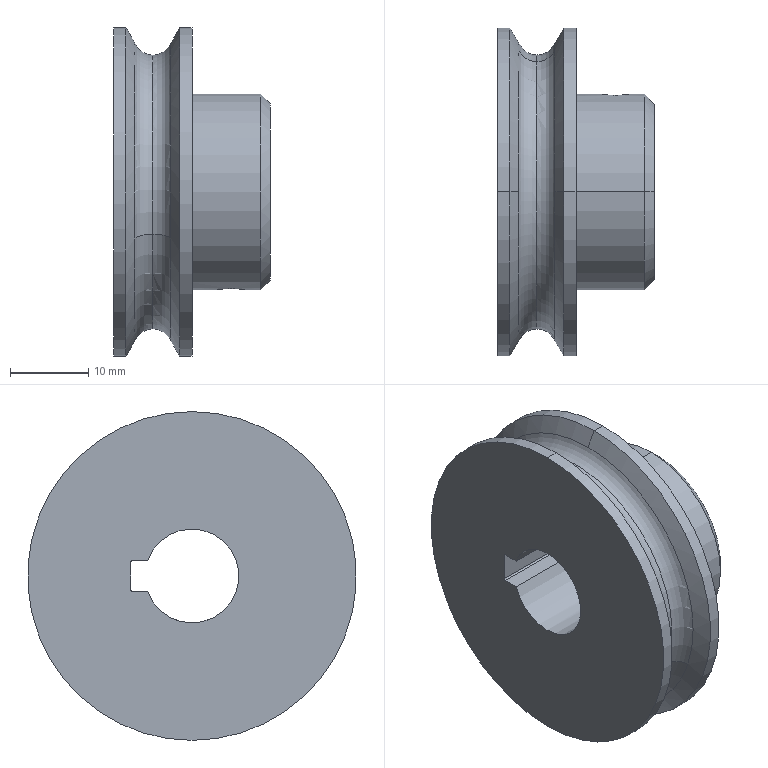Part | STEP file | MT-COMBO-119-S022 | 1 solid | 33 faces | box 20 x 42 x 42 mm | volume 14178 mm3 | cylinder 13 | cone 10 | plane 6 | torus 4 | commonest cylinder face diameters 3.242 x4 42 x4 0.4 x2 25 x2 12 x1
STEP:
#1=CARTESIAN_POINT('',(0.,16.643,5.408));
#2=VERTEX_POINT('',#1);
#3=CARTESIAN_POINT('',(2.299,18.087,5.877));
#4=VERTEX_POINT('',#3);
#5=CARTESIAN_POINT('',(0.,19.021,6.18));
#6=DIRECTION('',(0.,-0.309,0.9511));
#7=DIRECTION('',(-0.9196,-0.3736,-0.1214));
#8=AXIS2_PLACEMENT_3D('',#5,#6,#7);
#9=CIRCLE('',#8,2.5);
#10=EDGE_CURVE('',#2,#4,#9,.T.);
#11=ORIENTED_EDGE('',*,*,#10,.F.);
#12=CARTESIAN_POINT('',(0.,-16.643,-5.408));
#13=VERTEX_POINT('',#12);
#14=CARTESIAN_POINT('',(0.,0.,0.));
#15=DIRECTION('',(1.,0.,0.));
#16=DIRECTION('',(0.,0.,-1.));
#17=AXIS2_PLACEMENT_3D('',#14,#15,#16);
#18=CIRCLE('',#17,17.5);
#19=EDGE_CURVE('',#2,#13,#18,.T.);
#20=ORIENTED_EDGE('',*,*,#19,.T.);
#21=CARTESIAN_POINT('',(2.299,-18.087,-5.877));
#22=VERTEX_POINT('',#21);
#23=CARTESIAN_POINT('',(0.,-19.021,-6.18));
#24=DIRECTION('',(0.,0.309,-0.9511));
#25=DIRECTION('',(-0.9196,0.3736,0.1214));
#26=AXIS2_PLACEMENT_3D('',#23,#24,#25);
#27=CIRCLE('',#26,2.5);
#28=EDGE_CURVE('',#13,#22,#27,.T.);
#29=ORIENTED_EDGE('',*,*,#28,.T.);
#30=CARTESIAN_POINT('',(2.299,0.,19.018));
#31=VERTEX_POINT('',#30);
#32=CARTESIAN_POINT('',(2.299,0.,0.));
#33=DIRECTION('',(1.,0.,0.));
#34=DIRECTION('',(0.,0.,-1.));
#35=AXIS2_PLACEMENT_3D('',#32,#33,#34);
#36=CIRCLE('',#35,19.018);
#37=EDGE_CURVE('',#31,#22,#36,.T.);
#38=ORIENTED_EDGE('',*,*,#37,.F.);
#39=CARTESIAN_POINT('',(2.299,0.,0.));
#40=DIRECTION('',(1.,0.,0.));
#41=DIRECTION('',(0.,0.,-1.));
#42=AXIS2_PLACEMENT_3D('',#39,#40,#41);
#43=CIRCLE('',#42,19.018);
#44=EDGE_CURVE('',#4,#31,#43,.T.);
#45=ORIENTED_EDGE('',*,*,#44,.F.);
#46=EDGE_LOOP('',(#11,#20,#29,#38,#45));
#47=FACE_OUTER_BOUND('',#46,.T.);
#48=CARTESIAN_POINT('',(0.,0.,0.));
#49=DIRECTION('',(1.,0.,0.));
#50=DIRECTION('',(0.,0.309,-0.9511));
#51=AXIS2_PLACEMENT_3D('',#48,#49,#50);
#52=TOROIDAL_SURFACE('',#51,20.,2.5);
#53=ADVANCED_FACE('',(#47),#52,.F.);
#54=ORIENTED_EDGE('',*,*,#28,.F.);
#55=CARTESIAN_POINT('',(0.,0.,0.));
#56=DIRECTION('',(1.,0.,0.));
#57=DIRECTION('',(0.,0.,-1.));
#58=AXIS2_PLACEMENT_3D('',#55,#56,#57);
#59=CIRCLE('',#58,17.5);
#60=EDGE_CURVE('',#13,#2,#59,.T.);
#61=ORIENTED_EDGE('',*,*,#60,.T.);
#62=ORIENTED_EDGE('',*,*,#10,.T.);
#63=CARTESIAN_POINT('',(2.299,0.,-19.018));
#64=VERTEX_POINT('',#63);
#65=CARTESIAN_POINT('',(2.299,0.,0.));
#66=DIRECTION('',(1.,0.,0.));
#67=DIRECTION('',(0.,0.,-1.));
#68=AXIS2_PLACEMENT_3D('',#65,#66,#67);
#69=CIRCLE('',#68,19.018);
#70=EDGE_CURVE('',#64,#4,#69,.T.);
#71=ORIENTED_EDGE('',*,*,#70,.F.);
#72=CARTESIAN_POINT('',(2.299,0.,0.));
#73=DIRECTION('',(1.,0.,0.));
#74=DIRECTION('',(0.,0.,-1.));
#75=AXIS2_PLACEMENT_3D('',#72,#73,#74);
#76=CIRCLE('',#75,19.018);
#77=EDGE_CURVE('',#22,#64,#76,.T.);
#78=ORIENTED_EDGE('',*,*,#77,.F.);
#79=EDGE_LOOP('',(#54,#61,#62,#71,#78));
#80=FACE_OUTER_BOUND('',#79,.T.);
#81=CARTESIAN_POINT('',(0.,0.,0.));
#82=DIRECTION('',(1.,0.,0.));
#83=DIRECTION('',(0.,-0.309,0.9511));
#84=AXIS2_PLACEMENT_3D('',#81,#82,#83);
#85=TOROIDAL_SURFACE('',#84,20.,2.5);
#86=ADVANCED_FACE('',(#80),#85,.F.);
#87=CARTESIAN_POINT('',(5.,0.,12.5));
#88=VERTEX_POINT('',#87);
#89=CARTESIAN_POINT('',(13.75,0.,12.5));
#90=VERTEX_POINT('',#89);
#91=CARTESIAN_POINT('',(5.,0.,12.5));
#92=DIRECTION('',(1.,0.,0.));
#93=VECTOR('',#92,1000.);
#94=LINE('',#91,#93);
#95=EDGE_CURVE('',#88,#90,#94,.T.);
#96=ORIENTED_EDGE('',*,*,#95,.F.);
#97=CARTESIAN_POINT('',(5.,0.,-12.5));
#98=VERTEX_POINT('',#97);
#99=CARTESIAN_POINT('',(5.,0.,0.));
#100=DIRECTION('',(1.,0.,0.));
#101=DIRECTION('',(0.,0.,-1.));
#102=AXIS2_PLACEMENT_3D('',#99,#100,#101);
#103=CIRCLE('',#102,12.5);
#104=EDGE_CURVE('',#88,#98,#103,.T.);
#105=ORIENTED_EDGE('',*,*,#104,.T.);
#106=CARTESIAN_POINT('',(8.,0.,-12.5));
#107=VERTEX_POINT('',#106);
#108=CARTESIAN_POINT('',(5.,0.,-12.5));
#109=DIRECTION('',(1.,0.,0.));
#110=VECTOR('',#109,1000.);
#111=LINE('',#108,#110);
#112=EDGE_CURVE('',#98,#107,#111,.T.);
#113=ORIENTED_EDGE('',*,*,#112,.T.);
#114=CARTESIAN_POINT('',(8.634,-1.357,-12.426));
#115=VERTEX_POINT('',#114);
#116=CARTESIAN_POINT('',(8.,0.,-12.5));
#117=CARTESIAN_POINT('',(8.,-0.2576,-12.5));
#118=CARTESIAN_POINT('',(8.059,-0.5152,-12.492));
#119=CARTESIAN_POINT('',(8.28,-0.9815,-12.464));
#120=CARTESIAN_POINT('',(8.441,-1.189,-12.444));
#121=CARTESIAN_POINT('',(8.634,-1.357,-12.426));
#122=B_SPLINE_CURVE_WITH_KNOTS('',3,(#116,#117,#118,#119,#120,#121),.UNSPECIFIED.,.F.,.F.,(4,2,4),(0.8726,0.9363,1.),.UNSPECIFIED.);
#123=EDGE_CURVE('',#107,#115,#122,.T.);
#124=ORIENTED_EDGE('',*,*,#123,.T.);
#125=CARTESIAN_POINT('',(12.,0.,-12.5));
#126=VERTEX_POINT('',#125);
#127=CARTESIAN_POINT('',(8.634,-1.357,-12.426));
#128=CARTESIAN_POINT('',(8.916,-1.603,-12.399));
#129=CARTESIAN_POINT('',(9.272,-1.767,-12.375));
#130=CARTESIAN_POINT('',(10.014,-1.894,-12.356));
#131=CARTESIAN_POINT('',(10.402,-1.857,-12.362));
#132=CARTESIAN_POINT('',(10.931,-1.655,-12.39));
#133=CARTESIAN_POINT('',(11.098,-1.565,-12.402));
#134=CARTESIAN_POINT('',(11.399,-1.34,-12.429));
#135=CARTESIAN_POINT('',(11.535,-1.205,-12.443));
#136=CARTESIAN_POINT('',(11.758,-0.904,-12.468));
#137=CARTESIAN_POINT('',(11.848,-0.7339,-12.48));
#138=CARTESIAN_POINT('',(11.969,-0.3777,-12.496));
#139=CARTESIAN_POINT('',(12.,-0.1886,-12.5));
#140=CARTESIAN_POINT('',(12.,0.,-12.5));
#141=B_SPLINE_CURVE_WITH_KNOTS('',3,(#127,#128,#129,#130,#131,#132,#133,#134,#135,#136,#137,#138,#139,#140),.UNSPECIFIED.,.F.,.F.,(4,2,2,2,2,2,4),(0.,0.09314,0.1863,0.2328,0.2794,0.326,0.3726),.UNSPECIFIED.);
#142=EDGE_CURVE('',#115,#126,#141,.T.);
#143=ORIENTED_EDGE('',*,*,#142,.T.);
#144=CARTESIAN_POINT('',(13.75,0.,-12.5));
#145=VERTEX_POINT('',#144);
#146=CARTESIAN_POINT('',(12.,0.,-12.5));
#147=DIRECTION('',(1.,0.,0.));
#148=VECTOR('',#147,1000.);
#149=LINE('',#146,#148);
#150=EDGE_CURVE('',#126,#145,#149,.T.);
#151=ORIENTED_EDGE('',*,*,#150,.T.);
#152=CARTESIAN_POINT('',(13.75,0.,0.));
#153=DIRECTION('',(1.,0.,0.));
#154=DIRECTION('',(0.,0.,-1.));
#155=AXIS2_PLACEMENT_3D('',#152,#153,#154);
#156=CIRCLE('',#155,12.5);
#157=EDGE_CURVE('',#90,#145,#156,.T.);
#158=ORIENTED_EDGE('',*,*,#157,.F.);
#159=EDGE_LOOP('',(#96,#105,#113,#124,#143,#151,#158));
#160=FACE_OUTER_BOUND('',#159,.T.);
#161=CARTESIAN_POINT('',(15.,0.,0.));
#162=DIRECTION('',(1.,0.,0.));
#163=DIRECTION('',(0.,1.,0.));
#164=AXIS2_PLACEMENT_3D('',#161,#162,#163);
#165=CYLINDRICAL_SURFACE('',#164,12.5);
#166=ADVANCED_FACE('',(#160),#165,.T.);
#167=CARTESIAN_POINT('',(15.,0.,-11.25));
#168=VERTEX_POINT('',#167);
#169=CARTESIAN_POINT('',(15.,0.,-11.25));
#170=DIRECTION('',(-0.7071,0.,-0.7071));
#171=VECTOR('',#170,1000.);
#172=LINE('',#169,#171);
#173=EDGE_CURVE('',#168,#145,#172,.T.);
#174=ORIENTED_EDGE('',*,*,#173,.F.);
#175=CARTESIAN_POINT('',(15.,0.,11.25));
#176=VERTEX_POINT('',#175);
#177=CARTESIAN_POINT('',(15.,0.,0.));
#178=DIRECTION('',(1.,0.,0.));
#179=DIRECTION('',(0.,0.,-1.));
#180=AXIS2_PLACEMENT_3D('',#177,#178,#179);
#181=CIRCLE('',#180,11.25);
#182=EDGE_CURVE('',#176,#168,#181,.T.);
#183=ORIENTED_EDGE('',*,*,#182,.F.);
#184=CARTESIAN_POINT('',(15.,0.,11.25));
#185=DIRECTION('',(-0.7071,0.,0.7071));
#186=VECTOR('',#185,1000.);
#187=LINE('',#184,#186);
#188=EDGE_CURVE('',#176,#90,#187,.T.);
#189=ORIENTED_EDGE('',*,*,#188,.T.);
#190=ORIENTED_EDGE('',*,*,#157,.T.);
#191=EDGE_LOOP('',(#174,#183,#189,#190));
#192=FACE_OUTER_BOUND('',#191,.T.);
#193=CARTESIAN_POINT('',(15.,0.,0.));
#194=DIRECTION('',(-1.,0.,0.));
#195=DIRECTION('',(0.,1.,0.));
#196=AXIS2_PLACEMENT_3D('',#193,#194,#195);
#197=CONICAL_SURFACE('',#196,11.25,0.7854);
#198=ADVANCED_FACE('',(#192),#197,.T.);
#199=ORIENTED_EDGE('',*,*,#173,.T.);
#200=CARTESIAN_POINT('',(13.75,0.,0.));
#201=DIRECTION('',(1.,0.,0.));
#202=DIRECTION('',(0.,0.,-1.));
#203=AXIS2_PLACEMENT_3D('',#200,#201,#202);
#204=CIRCLE('',#203,12.5);
#205=EDGE_CURVE('',#145,#90,#204,.T.);
#206=ORIENTED_EDGE('',*,*,#205,.T.);
#207=ORIENTED_EDGE('',*,*,#188,.F.);
#208=CARTESIAN_POINT('',(15.,0.,0.));
#209=DIRECTION('',(1.,0.,0.));
#210=DIRECTION('',(0.,0.,-1.));
#211=AXIS2_PLACEMENT_3D('',#208,#209,#210);
#212=CIRCLE('',#211,11.25);
#213=EDGE_CURVE('',#168,#176,#212,.T.);
#214=ORIENTED_EDGE('',*,*,#213,.F.);
#215=EDGE_LOOP('',(#199,#206,#207,#214));
#216=FACE_OUTER_BOUND('',#215,.T.);
#217=CARTESIAN_POINT('',(15.,0.,0.));
#218=DIRECTION('',(-1.,0.,0.));
#219=DIRECTION('',(0.,-1.,0.));
#220=AXIS2_PLACEMENT_3D('',#217,#218,#219);
#221=CONICAL_SURFACE('',#220,11.25,0.7854);
#222=ADVANCED_FACE('',(#216),#221,.T.);
#223=ORIENTED_EDGE('',*,*,#213,.T.);
#224=ORIENTED_EDGE('',*,*,#182,.T.);
#225=EDGE_LOOP('',(#223,#224));
#226=FACE_OUTER_BOUND('',#225,.T.);
#227=CARTESIAN_POINT('',(15.,5.657,2.));
#228=VERTEX_POINT('',#227);
#229=CARTESIAN_POINT('',(15.,5.657,-2.));
#230=VERTEX_POINT('',#229);
#231=CARTESIAN_POINT('',(15.,0.,0.));
#232=DIRECTION('',(1.,0.,0.));
#233=DIRECTION('',(0.,0.,-1.));
#234=AXIS2_PLACEMENT_3D('',#231,#232,#233);
#235=CIRCLE('',#234,6.);
#236=EDGE_CURVE('',#228,#230,#235,.T.);
#237=ORIENTED_EDGE('',*,*,#236,.F.);
#238=CARTESIAN_POINT('',(15.,7.6,2.));
#239=VERTEX_POINT('',#238);
#240=CARTESIAN_POINT('',(15.,6.,2.));
#241=DIRECTION('',(0.,1.,0.));
#242=VECTOR('',#241,1000.);
#243=LINE('',#240,#242);
#244=EDGE_CURVE('',#228,#239,#243,.T.);
#245=ORIENTED_EDGE('',*,*,#244,.T.);
#246=CARTESIAN_POINT('',(15.,7.8,1.8));
#247=VERTEX_POINT('',#246);
#248=CARTESIAN_POINT('',(15.,7.6,1.8));
#249=DIRECTION('',(-1.,0.,0.));
#250=DIRECTION('',(0.,0.,-1.));
#251=AXIS2_PLACEMENT_3D('',#248,#249,#250);
#252=CIRCLE('',#251,0.2);
#253=EDGE_CURVE('',#239,#247,#252,.T.);
#254=ORIENTED_EDGE('',*,*,#253,.T.);
#255=CARTESIAN_POINT('',(15.,7.8,-1.8));
#256=VERTEX_POINT('',#255);
#257=CARTESIAN_POINT('',(15.,7.8,0.));
#258=DIRECTION('',(0.,0.,-1.));
#259=VECTOR('',#258,1000.);
#260=LINE('',#257,#259);
#261=EDGE_CURVE('',#247,#256,#260,.T.);
#262=ORIENTED_EDGE('',*,*,#261,.T.);
#263=CARTESIAN_POINT('',(15.,7.6,-2.));
#264=VERTEX_POINT('',#263);
#265=CARTESIAN_POINT('',(15.,7.6,-1.8));
#266=DIRECTION('',(-1.,0.,0.));
#267=DIRECTION('',(0.,0.,-1.));
#268=AXIS2_PLACEMENT_3D('',#265,#266,#267);
#269=CIRCLE('',#268,0.2);
#270=EDGE_CURVE('',#256,#264,#269,.T.);
#271=ORIENTED_EDGE('',*,*,#270,.T.);
#272=CARTESIAN_POINT('',(15.,6.,-2.));
#273=DIRECTION('',(0.,-1.,0.));
#274=VECTOR('',#273,1000.);
#275=LINE('',#272,#274);
#276=EDGE_CURVE('',#264,#230,#275,.T.);
#277=ORIENTED_EDGE('',*,*,#276,.T.);
#278=EDGE_LOOP('',(#237,#245,#254,#262,#271,#277));
#279=FACE_BOUND('',#278,.T.);
#280=CARTESIAN_POINT('',(15.,6.,0.));
#281=DIRECTION('',(1.,0.,0.));
#282=DIRECTION('',(0.,0.,-1.));
#283=AXIS2_PLACEMENT_3D('',#280,#281,#282);
#284=PLANE('',#283);
#285=ADVANCED_FACE('',(#226,#279),#284,.T.);
#286=ORIENTED_EDGE('',*,*,#276,.F.);
#287=CARTESIAN_POINT('',(-5.,7.6,-2.));
#288=VERTEX_POINT('',#287);
#289=CARTESIAN_POINT('',(25.,7.6,-2.));
#290=DIRECTION('',(-1.,0.,0.));
#291=VECTOR('',#290,1000.);
#292=LINE('',#289,#291);
#293=EDGE_CURVE('',#264,#288,#292,.T.);
#294=ORIENTED_EDGE('',*,*,#293,.T.);
#295=CARTESIAN_POINT('',(-5.,5.657,-2.));
#296=VERTEX_POINT('',#295);
#297=CARTESIAN_POINT('',(-5.,4.2,-2.));
#298=DIRECTION('',(0.,1.,0.));
#299=VECTOR('',#298,1000.);
#300=LINE('',#297,#299);
#301=EDGE_CURVE('',#296,#288,#300,.T.);
#302=ORIENTED_EDGE('',*,*,#301,.F.);
#303=CARTESIAN_POINT('',(15.,5.657,-2.));
#304=DIRECTION('',(-1.,0.,0.));
#305=VECTOR('',#304,1000.);
#306=LINE('',#303,#305);
#307=EDGE_CURVE('',#230,#296,#306,.T.);
#308=ORIENTED_EDGE('',*,*,#307,.F.);
#309=EDGE_LOOP('',(#286,#294,#302,#308));
#310=FACE_OUTER_BOUND('',#309,.T.);
#311=CARTESIAN_POINT('',(25.,4.2,-2.));
#312=DIRECTION('',(0.,0.,1.));
#313=DIRECTION('',(1.,0.,0.));
#314=AXIS2_PLACEMENT_3D('',#311,#312,#313);
#315=PLANE('',#314);
#316=ADVANCED_FACE('',(#310),#315,.T.);
#317=CARTESIAN_POINT('',(-5.,5.657,2.));
#318=VERTEX_POINT('',#317);
#319=CARTESIAN_POINT('',(-5.,0.,0.));
#320=DIRECTION('',(1.,0.,0.));
#321=DIRECTION('',(0.,0.,-1.));
#322=AXIS2_PLACEMENT_3D('',#319,#320,#321);
#323=CIRCLE('',#322,6.);
#324=EDGE_CURVE('',#318,#296,#323,.T.);
#325=ORIENTED_EDGE('',*,*,#324,.F.);
#326=CARTESIAN_POINT('',(15.,5.657,2.));
#327=DIRECTION('',(1.,0.,0.));
#328=VECTOR('',#327,1000.);
#329=LINE('',#326,#328);
#330=EDGE_CURVE('',#318,#228,#329,.T.);
#331=ORIENTED_EDGE('',*,*,#330,.T.);
#332=ORIENTED_EDGE('',*,*,#236,.T.);
#333=ORIENTED_EDGE('',*,*,#307,.T.);
#334=EDGE_LOOP('',(#325,#331,#332,#333));
#335=FACE_OUTER_BOUND('',#334,.T.);
#336=CARTESIAN_POINT('',(11.621,0.,-6.));
#337=VERTEX_POINT('',#336);
#338=CARTESIAN_POINT('',(8.379,0.,-6.));
#339=VERTEX_POINT('',#338);
#340=CARTESIAN_POINT('',(11.621,0.,-6.));
#341=CARTESIAN_POINT('',(11.621,-0.2122,-6.));
#342=CARTESIAN_POINT('',(11.578,-0.4261,-5.988));
#343=CARTESIAN_POINT('',(11.415,-0.8177,-5.947));
#344=CARTESIAN_POINT('',(11.296,-0.9965,-5.919));
#345=CARTESIAN_POINT('',(10.997,-1.296,-5.86));
#346=CARTESIAN_POINT('',(10.818,-1.415,-5.831));
#347=CARTESIAN_POINT('',(10.426,-1.578,-5.789));
#348=CARTESIAN_POINT('',(10.213,-1.621,-5.777));
#349=CARTESIAN_POINT('',(9.786,-1.621,-5.777));
#350=CARTESIAN_POINT('',(9.573,-1.578,-5.789));
#351=CARTESIAN_POINT('',(9.182,-1.416,-5.831));
#352=CARTESIAN_POINT('',(9.003,-1.296,-5.86));
#353=CARTESIAN_POINT('',(8.705,-0.9974,-5.918));
#354=CARTESIAN_POINT('',(8.585,-0.8186,-5.947));
#355=CARTESIAN_POINT('',(8.422,-0.4262,-5.988));
#356=CARTESIAN_POINT('',(8.379,-0.2137,-6.));
#357=CARTESIAN_POINT('',(8.379,0.,-6.));
#358=B_SPLINE_CURVE_WITH_KNOTS('',3,(#340,#341,#342,#343,#344,#345,#346,#347,#348,#349,#350,#351,#352,#353,#354,#355,#356,#357),.UNSPECIFIED.,.F.,.F.,(4,2,2,2,2,2,2,2,4),(0.,0.0625,0.125,0.1875,0.25,0.3125,0.375,0.4375,0.5),.UNSPECIFIED.);
#359=EDGE_CURVE('',#337,#339,#358,.T.);
#360=ORIENTED_EDGE('',*,*,#359,.T.);
#361=CARTESIAN_POINT('',(8.379,0.,-6.));
#362=CARTESIAN_POINT('',(8.379,0.2137,-6.));
#363=CARTESIAN_POINT('',(8.422,0.426,-5.988));
#364=CARTESIAN_POINT('',(8.585,0.8187,-5.947));
#365=CARTESIAN_POINT('',(8.705,0.9971,-5.919));
#366=CARTESIAN_POINT('',(9.003,1.296,-5.86));
#367=CARTESIAN_POINT('',(9.183,1.416,-5.831));
#368=CARTESIAN_POINT('',(9.573,1.578,-5.789));
#369=CARTESIAN_POINT('',(9.787,1.621,-5.777));
#370=CARTESIAN_POINT('',(10.213,1.621,-5.777));
#371=CARTESIAN_POINT('',(10.426,1.578,-5.789));
#372=CARTESIAN_POINT('',(10.818,1.415,-5.831));
#373=CARTESIAN_POINT('',(10.997,1.296,-5.86));
#374=CARTESIAN_POINT('',(11.296,0.9963,-5.919));
#375=CARTESIAN_POINT('',(11.415,0.8177,-5.947));
#376=CARTESIAN_POINT('',(11.579,0.4253,-5.988));
#377=CARTESIAN_POINT('',(11.621,0.2122,-6.));
#378=CARTESIAN_POINT('',(11.621,0.,-6.));
#379=B_SPLINE_CURVE_WITH_KNOTS('',3,(#361,#362,#363,#364,#365,#366,#367,#368,#369,#370,#371,#372,#373,#374,#375,#376,#377,#378),.UNSPECIFIED.,.F.,.F.,(4,2,2,2,2,2,2,2,4),(0.5,0.5625,0.625,0.6875,0.75,0.8125,0.875,0.9375,1.),.UNSPECIFIED.);
#380=EDGE_CURVE('',#339,#337,#379,.T.);
#381=ORIENTED_EDGE('',*,*,#380,.T.);
#382=EDGE_LOOP('',(#360,#381));
#383=FACE_BOUND('',#382,.T.);
#384=CARTESIAN_POINT('',(15.,0.,0.));
#385=DIRECTION('',(1.,0.,0.));
#386=DIRECTION('',(0.,1.,0.));
#387=AXIS2_PLACEMENT_3D('',#384,#385,#386);
#388=CYLINDRICAL_SURFACE('',#387,6.);
#389=ADVANCED_FACE('',(#335,#383),#388,.F.);
#390=CARTESIAN_POINT('',(8.379,0.,-12.121));
#391=VERTEX_POINT('',#390);
#392=CARTESIAN_POINT('',(8.379,0.,-12.121));
#393=DIRECTION('',(0.,0.,1.));
#394=VECTOR('',#393,1000.);
#395=LINE('',#392,#394);
#396=EDGE_CURVE('',#391,#339,#395,.T.);
#397=ORIENTED_EDGE('',*,*,#396,.F.);
#398=CARTESIAN_POINT('',(11.621,0.,-12.121));
#399=VERTEX_POINT('',#398);
#400=CARTESIAN_POINT('',(10.,0.,-12.121));
#401=DIRECTION('',(0.,0.,1.));
#402=DIRECTION('',(1.,0.,0.));
#403=AXIS2_PLACEMENT_3D('',#400,#401,#402);
#404=CIRCLE('',#403,1.621);
#405=EDGE_CURVE('',#399,#391,#404,.T.);
#406=ORIENTED_EDGE('',*,*,#405,.F.);
#407=CARTESIAN_POINT('',(11.621,0.,-12.121));
#408=DIRECTION('',(0.,0.,1.));
#409=VECTOR('',#408,1000.);
#410=LINE('',#407,#409);
#411=EDGE_CURVE('',#399,#337,#410,.T.);
#412=ORIENTED_EDGE('',*,*,#411,.T.);
#413=ORIENTED_EDGE('',*,*,#380,.F.);
#414=EDGE_LOOP('',(#397,#406,#412,#413));
#415=FACE_OUTER_BOUND('',#414,.T.);
#416=CARTESIAN_POINT('',(10.,0.,-5.));
#417=DIRECTION('',(0.,0.,1.));
#418=DIRECTION('',(0.,-1.,0.));
#419=AXIS2_PLACEMENT_3D('',#416,#417,#418);
#420=CYLINDRICAL_SURFACE('',#419,1.621);
#421=ADVANCED_FACE('',(#415),#420,.F.);
#422=ORIENTED_EDGE('',*,*,#396,.T.);
#423=ORIENTED_EDGE('',*,*,#359,.F.);
#424=ORIENTED_EDGE('',*,*,#411,.F.);
#425=CARTESIAN_POINT('',(10.,0.,-12.121));
#426=DIRECTION('',(0.,0.,1.));
#427=DIRECTION('',(1.,0.,0.));
#428=AXIS2_PLACEMENT_3D('',#425,#426,#427);
#429=CIRCLE('',#428,1.621);
#430=EDGE_CURVE('',#391,#399,#429,.T.);
#431=ORIENTED_EDGE('',*,*,#430,.F.);
#432=EDGE_LOOP('',(#422,#423,#424,#431));
#433=FACE_OUTER_BOUND('',#432,.T.);
#434=CARTESIAN_POINT('',(10.,0.,-5.));
#435=DIRECTION('',(0.,0.,1.));
#436=DIRECTION('',(0.,1.,0.));
#437=AXIS2_PLACEMENT_3D('',#434,#435,#436);
#438=CYLINDRICAL_SURFACE('',#437,1.621);
#439=ADVANCED_FACE('',(#433),#438,.F.);
#440=CARTESIAN_POINT('',(11.621,-0.000000002,-12.121));
#441=DIRECTION('',(0.7071,-0.000000001,-0.7071));
#442=VECTOR('',#441,1000.);
#443=LINE('',#440,#442);
#444=EDGE_CURVE('',#399,#126,#443,.T.);
#445=ORIENTED_EDGE('',*,*,#444,.T.);
#446=ORIENTED_EDGE('',*,*,#142,.F.);
#447=ORIENTED_EDGE('',*,*,#123,.F.);
#448=CARTESIAN_POINT('',(8.379,0.,-12.121));
#449=DIRECTION('',(-0.7071,0.,-0.7071));
#450=VECTOR('',#449,1000.);
#451=LINE('',#448,#450);
#452=EDGE_CURVE('',#391,#107,#451,.T.);
#453=ORIENTED_EDGE('',*,*,#452,.F.);
#454=ORIENTED_EDGE('',*,*,#430,.T.);
#455=EDGE_LOOP('',(#445,#446,#447,#453,#454));
#456=FACE_OUTER_BOUND('',#455,.T.);
#457=CARTESIAN_POINT('',(10.,0.,-12.5));
#458=DIRECTION('',(0.,0.,-1.));
#459=DIRECTION('',(-0.000000002,1.,0.));
#460=AXIS2_PLACEMENT_3D('',#457,#458,#459);
#461=CONICAL_SURFACE('',#460,2.,0.7854);
#462=ADVANCED_FACE('',(#456),#461,.F.);
#463=ORIENTED_EDGE('',*,*,#444,.F.);
#464=ORIENTED_EDGE('',*,*,#405,.T.);
#465=ORIENTED_EDGE('',*,*,#452,.T.);
#466=CARTESIAN_POINT('',(12.,0.,-12.5));
#467=CARTESIAN_POINT('',(12.,0.2531,-12.5));
#468=CARTESIAN_POINT('',(11.943,0.5058,-12.492));
#469=CARTESIAN_POINT('',(11.731,0.963,-12.465));
#470=CARTESIAN_POINT('',(11.576,1.169,-12.446));
#471=CARTESIAN_POINT('',(11.201,1.507,-12.41));
#472=CARTESIAN_POINT('',(10.981,1.638,-12.393));
#473=CARTESIAN_POINT('',(10.507,1.815,-12.368));
#474=CARTESIAN_POINT('',(10.254,1.86,-12.361));
#475=CARTESIAN_POINT('',(9.748,1.861,-12.361));
#476=CARTESIAN_POINT('',(9.495,1.816,-12.368));
#477=CARTESIAN_POINT('',(9.021,1.639,-12.392));
#478=CARTESIAN_POINT('',(8.801,1.507,-12.41));
#479=CARTESIAN_POINT('',(8.425,1.17,-12.446));
#480=CARTESIAN_POINT('',(8.269,0.9635,-12.465));
#481=CARTESIAN_POINT('',(8.057,0.5063,-12.492));
#482=CARTESIAN_POINT('',(8.,0.2527,-12.5));
#483=CARTESIAN_POINT('',(8.,0.,-12.5));
#484=B_SPLINE_CURVE_WITH_KNOTS('',3,(#466,#467,#468,#469,#470,#471,#472,#473,#474,#475,#476,#477,#478,#479,#480,#481,#482,#483),.UNSPECIFIED.,.F.,.F.,(4,2,2,2,2,2,2,2,4),(0.3726,0.4351,0.4976,0.5601,0.6226,0.6851,0.7476,0.8101,0.8726),.UNSPECIFIED.);
#485=EDGE_CURVE('',#126,#107,#484,.T.);
#486=ORIENTED_EDGE('',*,*,#485,.F.);
#487=EDGE_LOOP('',(#463,#464,#465,#486));
#488=FACE_OUTER_BOUND('',#487,.T.);
#489=CARTESIAN_POINT('',(10.,0.,-12.5));
#490=DIRECTION('',(0.,0.,-1.));
#491=DIRECTION('',(-0.000000001,-1.,0.));
#492=AXIS2_PLACEMENT_3D('',#489,#490,#491);
#493=CONICAL_SURFACE('',#492,2.,0.7854);
#494=ADVANCED_FACE('',(#488),#493,.F.);
#495=ORIENTED_EDGE('',*,*,#95,.T.);
#496=ORIENTED_EDGE('',*,*,#205,.F.);
#497=ORIENTED_EDGE('',*,*,#150,.F.);
#498=ORIENTED_EDGE('',*,*,#485,.T.);
#499=ORIENTED_EDGE('',*,*,#112,.F.);
#500=CARTESIAN_POINT('',(5.,0.,0.));
#501=DIRECTION('',(1.,0.,0.));
#502=DIRECTION('',(0.,0.,-1.));
#503=AXIS2_PLACEMENT_3D('',#500,#501,#502);
#504=CIRCLE('',#503,12.5);
#505=EDGE_CURVE('',#98,#88,#504,.T.);
#506=ORIENTED_EDGE('',*,*,#505,.T.);
#507=EDGE_LOOP('',(#495,#496,#497,#498,#499,#506));
#508=FACE_OUTER_BOUND('',#507,.T.);
#509=CARTESIAN_POINT('',(8.634,12.426,-1.357));
#510=VERTEX_POINT('',#509);
#511=CARTESIAN_POINT('',(10.,12.361,-1.861));
#512=VERTEX_POINT('',#511);
#513=CARTESIAN_POINT('',(8.634,12.426,-1.357));
#514=CARTESIAN_POINT('',(8.82,12.408,-1.52));
#515=CARTESIAN_POINT('',(9.037,12.391,-1.647));
#516=CARTESIAN_POINT('',(9.503,12.368,-1.817));
#517=CARTESIAN_POINT('',(9.751,12.361,-1.861));
#518=CARTESIAN_POINT('',(10.,12.361,-1.861));
#519=B_SPLINE_CURVE_WITH_KNOTS('',3,(#513,#514,#515,#516,#517,#518),.UNSPECIFIED.,.F.,.F.,(4,2,4),(0.,0.06136,0.1227),.UNSPECIFIED.);
#520=EDGE_CURVE('',#510,#512,#519,.T.);
#521=ORIENTED_EDGE('',*,*,#520,.T.);
#522=CARTESIAN_POINT('',(10.,12.361,1.861));
#523=VERTEX_POINT('',#522);
#524=CARTESIAN_POINT('',(10.,12.361,-1.861));
#525=CARTESIAN_POINT('',(10.253,12.361,-1.86));
#526=CARTESIAN_POINT('',(10.506,12.368,-1.816));
#527=CARTESIAN_POINT('',(10.98,12.393,-1.638));
#528=CARTESIAN_POINT('',(11.2,12.41,-1.507));
#529=CARTESIAN_POINT('',(11.576,12.446,-1.169));
#530=CARTESIAN_POINT('',(11.73,12.465,-0.9637));
#531=CARTESIAN_POINT('',(11.944,12.492,-0.5038));
#532=CARTESIAN_POINT('',(12.,12.5,-0.2515));
#533=CARTESIAN_POINT('',(12.,12.5,0.2546));
#534=CARTESIAN_POINT('',(11.943,12.492,0.5072));
#535=CARTESIAN_POINT('',(11.73,12.465,0.9642));
#536=CARTESIAN_POINT('',(11.576,12.446,1.17));
#537=CARTESIAN_POINT('',(11.199,12.41,1.507));
#538=CARTESIAN_POINT('',(10.98,12.392,1.638));
#539=CARTESIAN_POINT('',(10.506,12.368,1.816));
#540=CARTESIAN_POINT('',(10.253,12.361,1.86));
#541=CARTESIAN_POINT('',(10.,12.361,1.861));
#542=B_SPLINE_CURVE_WITH_KNOTS('',3,(#524,#525,#526,#527,#528,#529,#530,#531,#532,#533,#534,#535,#536,#537,#538,#539,#540,#541),.UNSPECIFIED.,.F.,.F.,(4,2,2,2,2,2,2,2,4),(0.1227,0.1852,0.2477,0.3102,0.3727,0.4352,0.4977,0.5601,0.6226),.UNSPECIFIED.);
#543=EDGE_CURVE('',#512,#523,#542,.T.);
#544=ORIENTED_EDGE('',*,*,#543,.T.);
#545=CARTESIAN_POINT('',(10.,12.361,1.861));
#546=CARTESIAN_POINT('',(9.618,12.361,1.861));
#547=CARTESIAN_POINT('',(9.237,12.377,1.757));
#548=CARTESIAN_POINT('',(8.747,12.415,1.46));
#549=CARTESIAN_POINT('',(8.598,12.429,1.338));
#550=CARTESIAN_POINT('',(8.343,12.456,1.056));
#551=CARTESIAN_POINT('',(8.235,12.469,0.8941));
#552=CARTESIAN_POINT('',(8.078,12.489,0.5478));
#553=CARTESIAN_POINT('',(8.027,12.496,0.3599));
#554=CARTESIAN_POINT('',(7.989,12.501,-0.01981));
#555=CARTESIAN_POINT('',(8.003,12.5,-0.2133));
#556=CARTESIAN_POINT('',(8.134,12.482,-0.7704));
#557=CARTESIAN_POINT('',(8.348,12.453,-1.108));
#558=CARTESIAN_POINT('',(8.634,12.426,-1.357));
#559=B_SPLINE_CURVE_WITH_KNOTS('',3,(#545,#546,#547,#548,#549,#550,#551,#552,#553,#554,#555,#556,#557,#558),.UNSPECIFIED.,.F.,.F.,(4,2,2,2,2,2,4),(0.6226,0.717,0.7641,0.8113,0.8585,0.9057,1.),.UNSPECIFIED.);
#560=EDGE_CURVE('',#523,#510,#559,.T.);
#561=ORIENTED_EDGE('',*,*,#560,.T.);
#562=EDGE_LOOP('',(#521,#544,#561));
#563=FACE_BOUND('',#562,.T.);
#564=CARTESIAN_POINT('',(15.,0.,0.));
#565=DIRECTION('',(1.,0.,0.));
#566=DIRECTION('',(0.,-1.,0.));
#567=AXIS2_PLACEMENT_3D('',#564,#565,#566);
#568=CYLINDRICAL_SURFACE('',#567,12.5);
#569=ADVANCED_FACE('',(#508,#563),#568,.T.);
#570=CARTESIAN_POINT('',(10.,12.121,-1.621));
#571=VERTEX_POINT('',#570);
#572=CARTESIAN_POINT('',(10.,12.121,-1.621));
#573=DIRECTION('',(0.,0.7071,-0.7071));
#574=VECTOR('',#573,1000.);
#575=LINE('',#572,#574);
#576=EDGE_CURVE('',#571,#512,#575,.T.);
#577=ORIENTED_EDGE('',*,*,#576,.T.);
#578=ORIENTED_EDGE('',*,*,#520,.F.);
#579=ORIENTED_EDGE('',*,*,#560,.F.);
#580=CARTESIAN_POINT('',(10.,12.121,1.621));
#581=VERTEX_POINT('',#580);
#582=CARTESIAN_POINT('',(10.,12.121,1.621));
#583=DIRECTION('',(0.,0.7071,0.7071));
#584=VECTOR('',#583,1000.);
#585=LINE('',#582,#584);
#586=EDGE_CURVE('',#581,#523,#585,.T.);
#587=ORIENTED_EDGE('',*,*,#586,.F.);
#588=CARTESIAN_POINT('',(10.,12.121,0.));
#589=DIRECTION('',(0.,-1.,0.));
#590=DIRECTION('',(0.,0.,-1.));
#591=AXIS2_PLACEMENT_3D('',#588,#589,#590);
#592=CIRCLE('',#591,1.621);
#593=EDGE_CURVE('',#581,#571,#592,.T.);
#594=ORIENTED_EDGE('',*,*,#593,.T.);
#595=EDGE_LOOP('',(#577,#578,#579,#587,#594));
#596=FACE_OUTER_BOUND('',#595,.T.);
#597=CARTESIAN_POINT('',(10.,12.5,0.));
#598=DIRECTION('',(0.,1.,0.));
#599=DIRECTION('',(1.,0.,0.));
#600=AXIS2_PLACEMENT_3D('',#597,#598,#599);
#601=CONICAL_SURFACE('',#600,2.,0.7854);
#602=ADVANCED_FACE('',(#596),#601,.F.);
#603=CARTESIAN_POINT('',(10.,7.8,1.621));
#604=VERTEX_POINT('',#603);
#605=CARTESIAN_POINT('',(10.,12.121,1.621));
#606=DIRECTION('',(0.,-1.,0.));
#607=VECTOR('',#606,1000.);
#608=LINE('',#605,#607);
#609=EDGE_CURVE('',#581,#604,#608,.T.);
#610=ORIENTED_EDGE('',*,*,#609,.T.);
#611=CARTESIAN_POINT('',(10.,7.8,-1.621));
#612=VERTEX_POINT('',#611);
#613=CARTESIAN_POINT('',(10.,7.8,0.));
#614=DIRECTION('',(0.,-1.,0.));
#615=DIRECTION('',(0.,0.,-1.));
#616=AXIS2_PLACEMENT_3D('',#613,#614,#615);
#617=CIRCLE('',#616,1.621);
#618=EDGE_CURVE('',#604,#612,#617,.T.);
#619=ORIENTED_EDGE('',*,*,#618,.T.);
#620=CARTESIAN_POINT('',(10.,12.121,-1.621));
#621=DIRECTION('',(0.,-1.,0.));
#622=VECTOR('',#621,1000.);
#623=LINE('',#620,#622);
#624=EDGE_CURVE('',#571,#612,#623,.T.);
#625=ORIENTED_EDGE('',*,*,#624,.F.);
#626=ORIENTED_EDGE('',*,*,#593,.F.);
#627=EDGE_LOOP('',(#610,#619,#625,#626));
#628=FACE_OUTER_BOUND('',#627,.T.);
#629=CARTESIAN_POINT('',(10.,7.8,0.));
#630=DIRECTION('',(0.,-1.,0.));
#631=DIRECTION('',(1.,0.,0.));
#632=AXIS2_PLACEMENT_3D('',#629,#630,#631);
#633=CYLINDRICAL_SURFACE('',#632,1.621);
#634=ADVANCED_FACE('',(#628),#633,.F.);
#635=ORIENTED_EDGE('',*,*,#609,.F.);
#636=CARTESIAN_POINT('',(10.,12.121,0.));
#637=DIRECTION('',(0.,-1.,0.));
#638=DIRECTION('',(0.,0.,-1.));
#639=AXIS2_PLACEMENT_3D('',#636,#637,#638);
#640=CIRCLE('',#639,1.621);
#641=EDGE_CURVE('',#571,#581,#640,.T.);
#642=ORIENTED_EDGE('',*,*,#641,.F.);
#643=ORIENTED_EDGE('',*,*,#624,.T.);
#644=CARTESIAN_POINT('',(10.,7.8,0.));
#645=DIRECTION('',(0.,-1.,0.));
#646=DIRECTION('',(0.,0.,-1.));
#647=AXIS2_PLACEMENT_3D('',#644,#645,#646);
#648=CIRCLE('',#647,1.621);
#649=EDGE_CURVE('',#612,#604,#648,.T.);
#650=ORIENTED_EDGE('',*,*,#649,.T.);
#651=EDGE_LOOP('',(#635,#642,#643,#650));
#652=FACE_OUTER_BOUND('',#651,.T.);
#653=CARTESIAN_POINT('',(10.,7.8,0.));
#654=DIRECTION('',(0.,-1.,0.));
#655=DIRECTION('',(-1.,0.,0.));
#656=AXIS2_PLACEMENT_3D('',#653,#654,#655);
#657=CYLINDRICAL_SURFACE('',#656,1.621);
#658=ADVANCED_FACE('',(#652),#657,.F.);
#659=ORIENTED_EDGE('',*,*,#618,.F.);
#660=ORIENTED_EDGE('',*,*,#649,.F.);
#661=EDGE_LOOP('',(#659,#660));
#662=FACE_BOUND('',#661,.T.);
#663=CARTESIAN_POINT('',(-5.,7.8,1.8));
#664=VERTEX_POINT('',#663);
#665=CARTESIAN_POINT('',(25.,7.8,1.8));
#666=DIRECTION('',(-1.,0.,0.));
#667=VECTOR('',#666,1000.);
#668=LINE('',#665,#667);
#669=EDGE_CURVE('',#247,#664,#668,.T.);
#670=ORIENTED_EDGE('',*,*,#669,.T.);
#671=CARTESIAN_POINT('',(-5.,7.8,-1.8));
#672=VERTEX_POINT('',#671);
#673=CARTESIAN_POINT('',(-5.,7.8,-1.8));
#674=DIRECTION('',(0.,0.,1.));
#675=VECTOR('',#674,1000.);
#676=LINE('',#673,#675);
#677=EDGE_CURVE('',#672,#664,#676,.T.);
#678=ORIENTED_EDGE('',*,*,#677,.F.);
#679=CARTESIAN_POINT('',(25.,7.8,-1.8));
#680=DIRECTION('',(-1.,0.,0.));
#681=VECTOR('',#680,1000.);
#682=LINE('',#679,#681);
#683=EDGE_CURVE('',#256,#672,#682,.T.);
#684=ORIENTED_EDGE('',*,*,#683,.F.);
#685=ORIENTED_EDGE('',*,*,#261,.F.);
#686=EDGE_LOOP('',(#670,#678,#684,#685));
#687=FACE_OUTER_BOUND('',#686,.T.);
#688=CARTESIAN_POINT('',(25.,7.8,-1.8));
#689=DIRECTION('',(0.,-1.,0.));
#690=DIRECTION('',(0.,0.,-1.));
#691=AXIS2_PLACEMENT_3D('',#688,#689,#690);
#692=PLANE('',#691);
#693=ADVANCED_FACE('',(#662,#687),#692,.T.);
#694=ORIENTED_EDGE('',*,*,#683,.T.);
#695=CARTESIAN_POINT('',(-5.,7.6,-1.8));
#696=DIRECTION('',(1.,0.,0.));
#697=DIRECTION('',(0.,0.,-1.));
#698=AXIS2_PLACEMENT_3D('',#695,#696,#697);
#699=CIRCLE('',#698,0.2);
#700=EDGE_CURVE('',#288,#672,#699,.T.);
#701=ORIENTED_EDGE('',*,*,#700,.F.);
#702=ORIENTED_EDGE('',*,*,#293,.F.);
#703=ORIENTED_EDGE('',*,*,#270,.F.);
#704=EDGE_LOOP('',(#694,#701,#702,#703));
#705=FACE_OUTER_BOUND('',#704,.T.);
#706=CARTESIAN_POINT('',(25.,7.6,-1.8));
#707=DIRECTION('',(-1.,0.,0.));
#708=DIRECTION('',(0.,-0.7071,0.7071));
#709=AXIS2_PLACEMENT_3D('',#706,#707,#708);
#710=CYLINDRICAL_SURFACE('',#709,0.2);
#711=ADVANCED_FACE('',(#705),#710,.F.);
#712=ORIENTED_EDGE('',*,*,#677,.T.);
#713=CARTESIAN_POINT('',(-5.,7.6,2.));
#714=VERTEX_POINT('',#713);
#715=CARTESIAN_POINT('',(-5.,7.6,1.8));
#716=DIRECTION('',(1.,0.,0.));
#717=DIRECTION('',(0.,0.,-1.));
#718=AXIS2_PLACEMENT_3D('',#715,#716,#717);
#719=CIRCLE('',#718,0.2);
#720=EDGE_CURVE('',#664,#714,#719,.T.);
#721=ORIENTED_EDGE('',*,*,#720,.T.);
#722=CARTESIAN_POINT('',(-5.,7.6,2.));
#723=DIRECTION('',(0.,-1.,0.));
#724=VECTOR('',#723,1000.);
#725=LINE('',#722,#724);
#726=EDGE_CURVE('',#714,#318,#725,.T.);
#727=ORIENTED_EDGE('',*,*,#726,.T.);
#728=ORIENTED_EDGE('',*,*,#324,.T.);
#729=ORIENTED_EDGE('',*,*,#301,.T.);
#730=ORIENTED_EDGE('',*,*,#700,.T.);
#731=EDGE_LOOP('',(#712,#721,#727,#728,#729,#730));
#732=FACE_BOUND('',#731,.T.);
#733=CARTESIAN_POINT('',(-5.,0.,21.));
#734=VERTEX_POINT('',#733);
#735=CARTESIAN_POINT('',(-5.,0.,-21.));
#736=VERTEX_POINT('',#735);
#737=CARTESIAN_POINT('',(-5.,0.,0.));
#738=DIRECTION('',(1.,0.,0.));
#739=DIRECTION('',(0.,0.,-1.));
#740=AXIS2_PLACEMENT_3D('',#737,#738,#739);
#741=CIRCLE('',#740,21.);
#742=EDGE_CURVE('',#734,#736,#741,.T.);
#743=ORIENTED_EDGE('',*,*,#742,.F.);
#744=CARTESIAN_POINT('',(-5.,0.,0.));
#745=DIRECTION('',(1.,0.,0.));
#746=DIRECTION('',(0.,0.,-1.));
#747=AXIS2_PLACEMENT_3D('',#744,#745,#746);
#748=CIRCLE('',#747,21.);
#749=EDGE_CURVE('',#736,#734,#748,.T.);
#750=ORIENTED_EDGE('',*,*,#749,.F.);
#751=EDGE_LOOP('',(#743,#750));
#752=FACE_OUTER_BOUND('',#751,.T.);
#753=CARTESIAN_POINT('',(-5.,21.,0.));
#754=DIRECTION('',(-1.,0.,0.));
#755=DIRECTION('',(0.,0.,1.));
#756=AXIS2_PLACEMENT_3D('',#753,#754,#755);
#757=PLANE('',#756);
#758=ADVANCED_FACE('',(#732,#752),#757,.T.);
#759=CARTESIAN_POINT('',(-3.443,0.,21.));
#760=VERTEX_POINT('',#759);
#761=CARTESIAN_POINT('',(-5.,0.,21.));
#762=DIRECTION('',(1.,0.,0.));
#763=VECTOR('',#762,1000.);
#764=LINE('',#761,#763);
#765=EDGE_CURVE('',#734,#760,#764,.T.);
#766=ORIENTED_EDGE('',*,*,#765,.T.);
#767=CARTESIAN_POINT('',(-3.443,0.,-21.));
#768=VERTEX_POINT('',#767);
#769=CARTESIAN_POINT('',(-3.443,0.,0.));
#770=DIRECTION('',(1.,0.,0.));
#771=DIRECTION('',(0.,0.,-1.));
#772=AXIS2_PLACEMENT_3D('',#769,#770,#771);
#773=CIRCLE('',#772,21.);
#774=EDGE_CURVE('',#768,#760,#773,.T.);
#775=ORIENTED_EDGE('',*,*,#774,.F.);
#776=CARTESIAN_POINT('',(-5.,0.,-21.));
#777=DIRECTION('',(1.,0.,0.));
#778=VECTOR('',#777,1000.);
#779=LINE('',#776,#778);
#780=EDGE_CURVE('',#736,#768,#779,.T.);
#781=ORIENTED_EDGE('',*,*,#780,.F.);
#782=ORIENTED_EDGE('',*,*,#749,.T.);
#783=EDGE_LOOP('',(#766,#775,#781,#782));
#784=FACE_OUTER_BOUND('',#783,.T.);
#785=CARTESIAN_POINT('',(15.,0.,0.));
#786=DIRECTION('',(1.,0.,0.));
#787=DIRECTION('',(0.,-1.,0.));
#788=AXIS2_PLACEMENT_3D('',#785,#786,#787);
#789=CYLINDRICAL_SURFACE('',#788,21.);
#790=ADVANCED_FACE('',(#784),#789,.T.);
#791=ORIENTED_EDGE('',*,*,#765,.F.);
#792=ORIENTED_EDGE('',*,*,#742,.T.);
#793=ORIENTED_EDGE('',*,*,#780,.T.);
#794=CARTESIAN_POINT('',(-3.443,0.,0.));
#795=DIRECTION('',(1.,0.,0.));
#796=DIRECTION('',(0.,0.,-1.));
#797=AXIS2_PLACEMENT_3D('',#794,#795,#796);
#798=CIRCLE('',#797,21.);
#799=EDGE_CURVE('',#760,#768,#798,.T.);
#800=ORIENTED_EDGE('',*,*,#799,.F.);
#801=EDGE_LOOP('',(#791,#792,#793,#800));
#802=FACE_OUTER_BOUND('',#801,.T.);
#803=CARTESIAN_POINT('',(15.,0.,0.));
#804=DIRECTION('',(1.,0.,0.));
#805=DIRECTION('',(0.,1.,0.));
#806=AXIS2_PLACEMENT_3D('',#803,#804,#805);
#807=CYLINDRICAL_SURFACE('',#806,21.);
#808=ADVANCED_FACE('',(#802),#807,.T.);
#809=CARTESIAN_POINT('',(-2.299,0.,-19.018));
#810=VERTEX_POINT('',#809);
#811=CARTESIAN_POINT('',(-2.299,0.,-19.018));
#812=DIRECTION('',(-0.5,0.,-0.866));
#813=VECTOR('',#812,1000.);
#814=LINE('',#811,#813);
#815=EDGE_CURVE('',#810,#768,#814,.T.);
#816=ORIENTED_EDGE('',*,*,#815,.F.);
#817=CARTESIAN_POINT('',(-2.299,-18.087,-5.877));
#818=VERTEX_POINT('',#817);
#819=CARTESIAN_POINT('',(-2.299,0.,0.));
#820=DIRECTION('',(1.,0.,0.));
#821=DIRECTION('',(0.,0.,-1.));
#822=AXIS2_PLACEMENT_3D('',#819,#820,#821);
#823=CIRCLE('',#822,19.018);
#824=EDGE_CURVE('',#818,#810,#823,.T.);
#825=ORIENTED_EDGE('',*,*,#824,.F.);
#826=CARTESIAN_POINT('',(-2.299,0.,19.018));
#827=VERTEX_POINT('',#826);
#828=CARTESIAN_POINT('',(-2.299,0.,0.));
#829=DIRECTION('',(1.,0.,0.));
#830=DIRECTION('',(0.,0.,-1.));
#831=AXIS2_PLACEMENT_3D('',#828,#829,#830);
#832=CIRCLE('',#831,19.018);
#833=EDGE_CURVE('',#827,#818,#832,.T.);
#834=ORIENTED_EDGE('',*,*,#833,.F.);
#835=CARTESIAN_POINT('',(-2.299,0.,19.018));
#836=DIRECTION('',(-0.5,0.,0.866));
#837=VECTOR('',#836,1000.);
#838=LINE('',#835,#837);
#839=EDGE_CURVE('',#827,#760,#838,.T.);
#840=ORIENTED_EDGE('',*,*,#839,.T.);
#841=ORIENTED_EDGE('',*,*,#799,.T.);
#842=EDGE_LOOP('',(#816,#825,#834,#840,#841));
#843=FACE_OUTER_BOUND('',#842,.T.);
#844=CARTESIAN_POINT('',(-2.299,0.,0.));
#845=DIRECTION('',(-1.,0.,0.));
#846=DIRECTION('',(0.,1.,0.));
#847=AXIS2_PLACEMENT_3D('',#844,#845,#846);
#848=CONICAL_SURFACE('',#847,19.018,1.047);
#849=ADVANCED_FACE('',(#843),#848,.T.);
#850=ORIENTED_EDGE('',*,*,#815,.T.);
#851=ORIENTED_EDGE('',*,*,#774,.T.);
#852=ORIENTED_EDGE('',*,*,#839,.F.);
#853=CARTESIAN_POINT('',(-2.299,18.087,5.877));
#854=VERTEX_POINT('',#853);
#855=CARTESIAN_POINT('',(-2.299,0.,0.));
#856=DIRECTION('',(1.,0.,0.));
#857=DIRECTION('',(0.,0.,-1.));
#858=AXIS2_PLACEMENT_3D('',#855,#856,#857);
#859=CIRCLE('',#858,19.018);
#860=EDGE_CURVE('',#854,#827,#859,.T.);
#861=ORIENTED_EDGE('',*,*,#860,.F.);
#862=CARTESIAN_POINT('',(-2.299,0.,0.));
#863=DIRECTION('',(1.,0.,0.));
#864=DIRECTION('',(0.,0.,-1.));
#865=AXIS2_PLACEMENT_3D('',#862,#863,#864);
#866=CIRCLE('',#865,19.018);
#867=EDGE_CURVE('',#810,#854,#866,.T.);
#868=ORIENTED_EDGE('',*,*,#867,.F.);
#869=EDGE_LOOP('',(#850,#851,#852,#861,#868));
#870=FACE_OUTER_BOUND('',#869,.T.);
#871=CARTESIAN_POINT('',(-2.299,0.,0.));
#872=DIRECTION('',(-1.,0.,0.));
#873=DIRECTION('',(0.,-1.,0.));
#874=AXIS2_PLACEMENT_3D('',#871,#872,#873);
#875=CONICAL_SURFACE('',#874,19.018,1.047);
#876=ADVANCED_FACE('',(#870),#875,.T.);
#877=ORIENTED_EDGE('',*,*,#60,.F.);
#878=CARTESIAN_POINT('',(0.,-19.021,-6.18));
#879=DIRECTION('',(0.,0.309,-0.9511));
#880=DIRECTION('',(-0.9196,0.3736,0.1214));
#881=AXIS2_PLACEMENT_3D('',#878,#879,#880);
#882=CIRCLE('',#881,2.5);
#883=EDGE_CURVE('',#818,#13,#882,.T.);
#884=ORIENTED_EDGE('',*,*,#883,.F.);
#885=ORIENTED_EDGE('',*,*,#824,.T.);
#886=ORIENTED_EDGE('',*,*,#867,.T.);
#887=CARTESIAN_POINT('',(0.,19.021,6.18));
#888=DIRECTION('',(0.,-0.309,0.9511));
#889=DIRECTION('',(-0.9196,-0.3736,-0.1214));
#890=AXIS2_PLACEMENT_3D('',#887,#888,#889);
#891=CIRCLE('',#890,2.5);
#892=EDGE_CURVE('',#854,#2,#891,.T.);
#893=ORIENTED_EDGE('',*,*,#892,.T.);
#894=EDGE_LOOP('',(#877,#884,#885,#886,#893));
#895=FACE_OUTER_BOUND('',#894,.T.);
#896=CARTESIAN_POINT('',(0.,0.,0.));
#897=DIRECTION('',(1.,0.,0.));
#898=DIRECTION('',(0.,-0.309,0.9511));
#899=AXIS2_PLACEMENT_3D('',#896,#897,#898);
#900=TOROIDAL_SURFACE('',#899,20.,2.5);
#901=ADVANCED_FACE('',(#895),#900,.F.);
#902=CARTESIAN_POINT('',(3.443,0.,21.));
#903=VERTEX_POINT('',#902);
#904=CARTESIAN_POINT('',(2.299,0.,19.018));
#905=DIRECTION('',(0.5,0.,0.866));
#906=VECTOR('',#905,1000.);
#907=LINE('',#904,#906);
#908=EDGE_CURVE('',#31,#903,#907,.T.);
#909=ORIENTED_EDGE('',*,*,#908,.F.);
#910=ORIENTED_EDGE('',*,*,#37,.T.);
#911=ORIENTED_EDGE('',*,*,#77,.T.);
#912=CARTESIAN_POINT('',(3.443,0.,-21.));
#913=VERTEX_POINT('',#912);
#914=CARTESIAN_POINT('',(2.299,0.,-19.018));
#915=DIRECTION('',(0.5,0.,-0.866));
#916=VECTOR('',#915,1000.);
#917=LINE('',#914,#916);
#918=EDGE_CURVE('',#64,#913,#917,.T.);
#919=ORIENTED_EDGE('',*,*,#918,.T.);
#920=CARTESIAN_POINT('',(3.443,0.,0.));
#921=DIRECTION('',(1.,0.,0.));
#922=DIRECTION('',(0.,0.,-1.));
#923=AXIS2_PLACEMENT_3D('',#920,#921,#922);
#924=CIRCLE('',#923,21.);
#925=EDGE_CURVE('',#903,#913,#924,.T.);
#926=ORIENTED_EDGE('',*,*,#925,.F.);
#927=EDGE_LOOP('',(#909,#910,#911,#919,#926));
#928=FACE_OUTER_BOUND('',#927,.T.);
#929=CARTESIAN_POINT('',(3.443,0.,0.));
#930=DIRECTION('',(1.,0.,0.));
#931=DIRECTION('',(0.,1.,0.));
#932=AXIS2_PLACEMENT_3D('',#929,#930,#931);
#933=CONICAL_SURFACE('',#932,21.,1.047);
#934=ADVANCED_FACE('',(#928),#933,.T.);
#935=CARTESIAN_POINT('',(5.,0.,21.));
#936=VERTEX_POINT('',#935);
#937=CARTESIAN_POINT('',(3.443,0.,21.));
#938=DIRECTION('',(1.,0.,0.));
#939=VECTOR('',#938,1000.);
#940=LINE('',#937,#939);
#941=EDGE_CURVE('',#903,#936,#940,.T.);
#942=ORIENTED_EDGE('',*,*,#941,.F.);
#943=ORIENTED_EDGE('',*,*,#925,.T.);
#944=CARTESIAN_POINT('',(5.,0.,-21.));
#945=VERTEX_POINT('',#944);
#946=CARTESIAN_POINT('',(3.443,0.,-21.));
#947=DIRECTION('',(1.,0.,0.));
#948=VECTOR('',#947,1000.);
#949=LINE('',#946,#948);
#950=EDGE_CURVE('',#913,#945,#949,.T.);
#951=ORIENTED_EDGE('',*,*,#950,.T.);
#952=CARTESIAN_POINT('',(5.,0.,0.));
#953=DIRECTION('',(1.,0.,0.));
#954=DIRECTION('',(0.,0.,-1.));
#955=AXIS2_PLACEMENT_3D('',#952,#953,#954);
#956=CIRCLE('',#955,21.);
#957=EDGE_CURVE('',#936,#945,#956,.T.);
#958=ORIENTED_EDGE('',*,*,#957,.F.);
#959=EDGE_LOOP('',(#942,#943,#951,#958));
#960=FACE_OUTER_BOUND('',#959,.T.);
#961=CARTESIAN_POINT('',(15.,0.,0.));
#962=DIRECTION('',(1.,0.,0.));
#963=DIRECTION('',(0.,1.,0.));
#964=AXIS2_PLACEMENT_3D('',#961,#962,#963);
#965=CYLINDRICAL_SURFACE('',#964,21.);
#966=ADVANCED_FACE('',(#960),#965,.T.);
#967=CARTESIAN_POINT('',(5.,0.,0.));
#968=DIRECTION('',(1.,0.,0.));
#969=DIRECTION('',(0.,0.,-1.));
#970=AXIS2_PLACEMENT_3D('',#967,#968,#969);
#971=CIRCLE('',#970,21.);
#972=EDGE_CURVE('',#945,#936,#971,.T.);
#973=ORIENTED_EDGE('',*,*,#972,.T.);
#974=ORIENTED_EDGE('',*,*,#957,.T.);
#975=EDGE_LOOP('',(#973,#974));
#976=FACE_OUTER_BOUND('',#975,.T.);
#977=ORIENTED_EDGE('',*,*,#104,.F.);
#978=ORIENTED_EDGE('',*,*,#505,.F.);
#979=EDGE_LOOP('',(#977,#978));
#980=FACE_BOUND('',#979,.T.);
#981=CARTESIAN_POINT('',(5.,12.5,0.));
#982=DIRECTION('',(1.,0.,0.));
#983=DIRECTION('',(0.,0.,-1.));
#984=AXIS2_PLACEMENT_3D('',#981,#982,#983);
#985=PLANE('',#984);
#986=ADVANCED_FACE('',(#976,#980),#985,.T.);
#987=ORIENTED_EDGE('',*,*,#941,.T.);
#988=ORIENTED_EDGE('',*,*,#972,.F.);
#989=ORIENTED_EDGE('',*,*,#950,.F.);
#990=CARTESIAN_POINT('',(3.443,0.,0.));
#991=DIRECTION('',(1.,0.,0.));
#992=DIRECTION('',(0.,0.,-1.));
#993=AXIS2_PLACEMENT_3D('',#990,#991,#992);
#994=CIRCLE('',#993,21.);
#995=EDGE_CURVE('',#913,#903,#994,.T.);
#996=ORIENTED_EDGE('',*,*,#995,.T.);
#997=EDGE_LOOP('',(#987,#988,#989,#996));
#998=FACE_OUTER_BOUND('',#997,.T.);
#999=CARTESIAN_POINT('',(15.,0.,0.));
#1000=DIRECTION('',(1.,0.,0.));
#1001=DIRECTION('',(0.,-1.,0.));
#1002=AXIS2_PLACEMENT_3D('',#999,#1000,#1001);
#1003=CYLINDRICAL_SURFACE('',#1002,21.);
#1004=ADVANCED_FACE('',(#998),#1003,.T.);
#1005=ORIENTED_EDGE('',*,*,#908,.T.);
#1006=ORIENTED_EDGE('',*,*,#995,.F.);
#1007=ORIENTED_EDGE('',*,*,#918,.F.);
#1008=ORIENTED_EDGE('',*,*,#70,.T.);
#1009=ORIENTED_EDGE('',*,*,#44,.T.);
#1010=EDGE_LOOP('',(#1005,#1006,#1007,#1008,#1009));
#1011=FACE_OUTER_BOUND('',#1010,.T.);
#1012=CARTESIAN_POINT('',(3.443,0.,0.));
#1013=DIRECTION('',(1.,0.,0.));
#1014=DIRECTION('',(0.,-1.,0.));
#1015=AXIS2_PLACEMENT_3D('',#1012,#1013,#1014);
#1016=CONICAL_SURFACE('',#1015,21.,1.047);
#1017=ADVANCED_FACE('',(#1011),#1016,.T.);
#1018=ORIENTED_EDGE('',*,*,#19,.F.);
#1019=ORIENTED_EDGE('',*,*,#892,.F.);
#1020=ORIENTED_EDGE('',*,*,#860,.T.);
#1021=ORIENTED_EDGE('',*,*,#833,.T.);
#1022=ORIENTED_EDGE('',*,*,#883,.T.);
#1023=EDGE_LOOP('',(#1018,#1019,#1020,#1021,#1022));
#1024=FACE_OUTER_BOUND('',#1023,.T.);
#1025=CARTESIAN_POINT('',(0.,0.,0.));
#1026=DIRECTION('',(1.,0.,0.));
#1027=DIRECTION('',(0.,0.309,-0.9511));
#1028=AXIS2_PLACEMENT_3D('',#1025,#1026,#1027);
#1029=TOROIDAL_SURFACE('',#1028,20.,2.5);
#1030=ADVANCED_FACE('',(#1024),#1029,.F.);
#1031=ORIENTED_EDGE('',*,*,#726,.F.);
#1032=CARTESIAN_POINT('',(25.,7.6,2.));
#1033=DIRECTION('',(-1.,0.,0.));
#1034=VECTOR('',#1033,1000.);
#1035=LINE('',#1032,#1034);
#1036=EDGE_CURVE('',#239,#714,#1035,.T.);
#1037=ORIENTED_EDGE('',*,*,#1036,.F.);
#1038=ORIENTED_EDGE('',*,*,#244,.F.);
#1039=ORIENTED_EDGE('',*,*,#330,.F.);
#1040=EDGE_LOOP('',(#1031,#1037,#1038,#1039));
#1041=FACE_OUTER_BOUND('',#1040,.T.);
#1042=CARTESIAN_POINT('',(25.,7.6,2.));
#1043=DIRECTION('',(0.,0.,-1.));
#1044=DIRECTION('',(-1.,0.,0.));
#1045=AXIS2_PLACEMENT_3D('',#1042,#1043,#1044);
#1046=PLANE('',#1045);
#1047=ADVANCED_FACE('',(#1041),#1046,.T.);
#1048=ORIENTED_EDGE('',*,*,#1036,.T.);
#1049=ORIENTED_EDGE('',*,*,#720,.F.);
#1050=ORIENTED_EDGE('',*,*,#669,.F.);
#1051=ORIENTED_EDGE('',*,*,#253,.F.);
#1052=EDGE_LOOP('',(#1048,#1049,#1050,#1051));
#1053=FACE_OUTER_BOUND('',#1052,.T.);
#1054=CARTESIAN_POINT('',(25.,7.6,1.8));
#1055=DIRECTION('',(-1.,0.,0.));
#1056=DIRECTION('',(0.,-0.7071,-0.7071));
#1057=AXIS2_PLACEMENT_3D('',#1054,#1055,#1056);
#1058=CYLINDRICAL_SURFACE('',#1057,0.2);
#1059=ADVANCED_FACE('',(#1053),#1058,.F.);
#1060=ORIENTED_EDGE('',*,*,#576,.F.);
#1061=ORIENTED_EDGE('',*,*,#641,.T.);
#1062=ORIENTED_EDGE('',*,*,#586,.T.);
#1063=ORIENTED_EDGE('',*,*,#543,.F.);
#1064=EDGE_LOOP('',(#1060,#1061,#1062,#1063));
#1065=FACE_OUTER_BOUND('',#1064,.T.);
#1066=CARTESIAN_POINT('',(10.,12.5,0.));
#1067=DIRECTION('',(0.,1.,0.));
#1068=DIRECTION('',(-1.,0.,0.));
#1069=AXIS2_PLACEMENT_3D('',#1066,#1067,#1068);
#1070=CONICAL_SURFACE('',#1069,2.,0.7854);
#1071=ADVANCED_FACE('',(#1065),#1070,.F.);
#1072=CLOSED_SHELL('',(#53,#86,#166,#198,#222,#285,#316,#389,#421,#439,#462,#494,#569,#602,#634,#658,#693,#711,#758,#790,#808,#849,#876,#901,#934,#966,#986,#1004,#1017,#1030,#1047,#1059,#1071));
#1073=MANIFOLD_SOLID_BREP('',#1072);
#1074=CARTESIAN_POINT('',(0.,0.,0.));
#1075=DIRECTION('',(0.,0.,1.));
#1076=DIRECTION('',(1.,0.,0.));
#1077=AXIS2_PLACEMENT_3D('',#1074,#1075,#1076);
#1078=(LENGTH_UNIT()NAMED_UNIT(*)SI_UNIT(.MILLI.,.METRE.));
#1079=UNCERTAINTY_MEASURE_WITH_UNIT(LENGTH_MEASURE(0.00001),#1078,'','');
#1080=(NAMED_UNIT(*)PLANE_ANGLE_UNIT()SI_UNIT($,.RADIAN.));
#1081=(NAMED_UNIT(*)SI_UNIT($,.STERADIAN.)SOLID_ANGLE_UNIT());
#1082=(GEOMETRIC_REPRESENTATION_CONTEXT(3)GLOBAL_UNCERTAINTY_ASSIGNED_CONTEXT((#1079))GLOBAL_UNIT_ASSIGNED_CONTEXT((#1078,#1080,#1081))REPRESENTATION_CONTEXT('',''));
#1083=ADVANCED_BREP_SHAPE_REPRESENTATION('',(#1073,#1077),#1082);